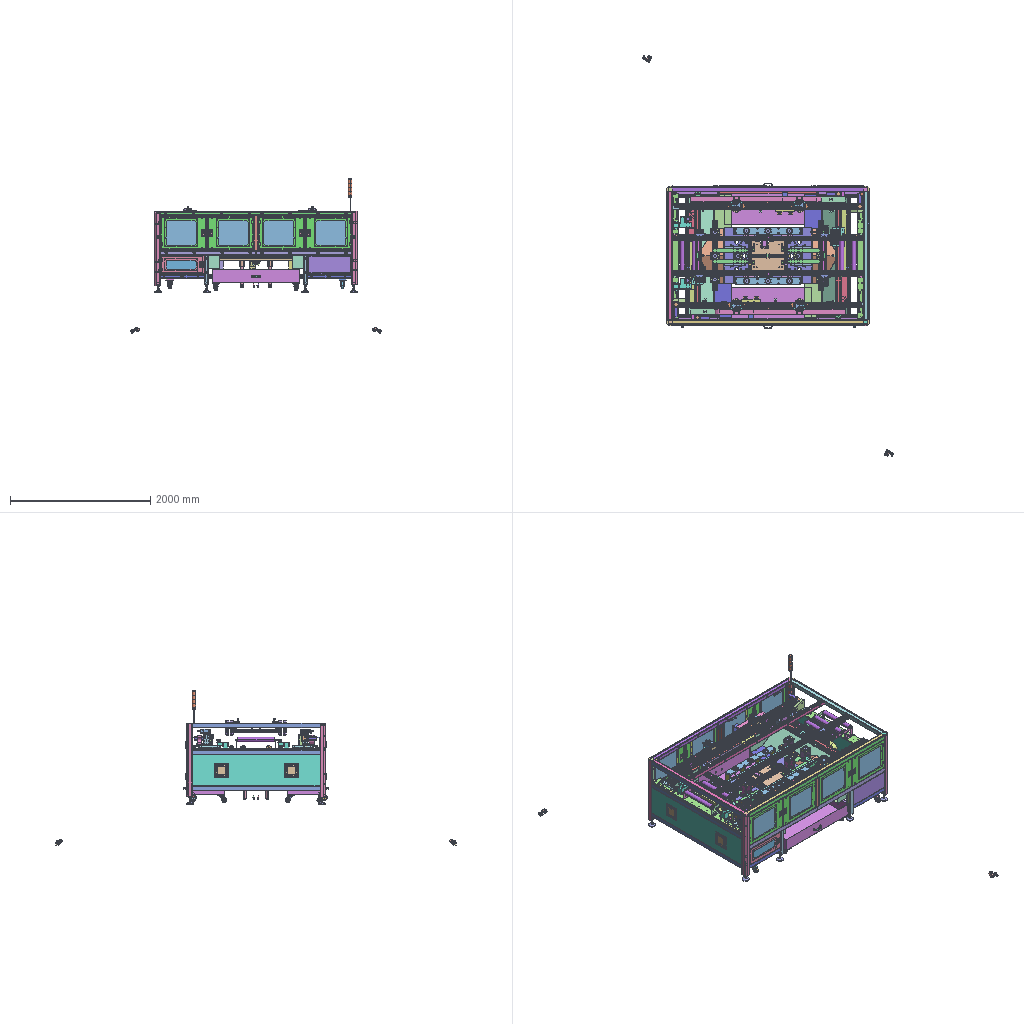Assembly | SolidWorks | 246 different items | 1119 placed | box 3582 x 5733 x 2213 mm
Parts list (item | name | quantity | parent item | size | volume | features):
1 | (subassembly) | x12 | in 4, 42 | 30 x 63 x 50 mm | 11600 mm3 | -
2 | (subassembly) | x4 | in 42 | 650 x 120 x 55.5 mm | 1855069 mm3 | features CompositeCurve 2
3 | (subassembly) | x1 | - | - | 84353797 mm3 | -
4 | (subassembly) | x2 | in 3 | - | 30075054 mm3 | features ReferencePattern 10, LocalLPattern 3, MirrorCompFeat 1
5 | (subassembly) | x2 | in 4 | 249.5 x 142 x 2600 mm | 14332524 mm3 | -
6 | (subassembly) | x2 | in 4 | 270 x 295.093 x 105 mm | 1190493 mm3 | features ReferencePattern 4, MirrorCompFeat 2
7 | (subassembly) | x4 | in 4 | 139.525 x 248.451 x 255.389 mm | 1113097 mm3 | -
8 | (subassembly) | x2 | in 3 | 1950 x 150 x 55.5 mm | 5101027 mm3 | features ReferencePattern 5, LocalLPattern 2, MirrorCompFeat 1
9 | (subassembly) | x2 | in 3 | 410 x 159.5 x 631 mm | 6148104 mm3 | features ReferencePattern 8, LocalLPattern 1, MirrorCompFeat 1
10 | (subassembly) | x2 | in 3 | 182.598 x 320 x 130 mm | 852374 mm3 | features CompositeCurve 6
11 | (subassembly) | x1 | - | - | 89338303 mm3 | features CompositeCurve 5, ReferencePattern 4, LocalLPattern 1
12 | (subassembly) | x1 | - | - | 55171435 mm3 | features ReferencePattern 18, MirrorCompFeat 9
13 | (subassembly) | x2 | in 12 | 953 x 227 x 231.5 mm | 4552776 mm3 | features ReferencePattern 11, MirrorCompFeat 2, CompositeCurve 1, LocalLPattern 1
14 | (subassembly) | x2 | in 12 | 100 x 125 x 230.841 mm | 827561 mm3 | -
15 | (subassembly) | x1 | in 12 | - | 34812843 mm3 | -
16 | (subassembly) | x1 | in 15 | - | 11539429 mm3 | features ReferencePattern 4, MirrorCompFeat 3, CompositeCurve 1, LocalLPattern 1
17 | (subassembly) | x4 | in 16 | 190 x 97 x 61 mm | 476303 mm3 | features CompositeCurve 1
18 | (subassembly) | x1 | in 15 | 1250 x 536.5 x 800 mm | 23012589 mm3 | features ReferencePattern 6, MirrorCompFeat 2, LocalLPattern 1
19 | (subassembly) | x2 | in 12 | 542.5 x 231.5 x 1000 mm | 4307591 mm3 | features ReferencePattern 11, LocalLPattern 2, MirrorCompFeat 2
20 | (subassembly) | x6 | in 19 | 125 x 100 x 191.5 mm | 742164 mm3 | -
21 | (subassembly) | x1 | - | - | 11952575 mm3 | features ReferencePattern 36, MirrorCompFeat 3, CompositeCurve 2, LocalLPattern 2
22 | (subassembly) | x2 | in 11 | 496 x 60 x 123 mm | 328404 mm3 | features MirrorCompFeat 3, ReferencePattern 3
23 | (subassembly) | x4 | in 21 | 110 x 69 x 42 mm | 113289 mm3 | -
24 | (subassembly) | x20 | in 33, 39 | 20.733 x 18.957 x 75.5 mm | 4578 mm3 | -
25 | (subassembly) | x8 | in 11 | 100 x 168 x 100 mm | 182730 mm3 | -
26 | (subassembly) | x8 | in 40 | 100 x 118 x 127 mm | 289275 mm3 | -
27 | (subassembly) | x2 | in 42 | 249.5 x 90 x 1730 mm | 9701440 mm3 | -
28 | (subassembly) | x8 | in 6, 43 | 118 x 54.3 x 21.2 mm | 85401 mm3 | -
29 | (subassembly) | x4 | in 7 | 177 x 112 x 48 mm | 579896 mm3 | features CompositeCurve 1
30 | (subassembly) | x2 | in 10 | 42 x 93.165 x 114.867 mm | 308752 mm3 | -
31 | (subassembly) | x12 | in 13, 19 | 51.5 x 67 x 13 mm | 7718 mm3 | -
32 | (subassembly) | x1 | in 18 | 421 x 93 x 190.924 mm | 447308 mm3 | -
33 | (subassembly) | x8 | in 11 | 670.712 x 493 x 25 mm | 1584341 mm3 | features MirrorCompFeat 1, ReferencePattern 1
34 | (subassembly) | x1 | in 16 | 137.5 x 90 x 275 mm | 2048513 mm3 | -
35 | (subassembly) | x4 | in 21 | 21 x 58.38 x 21 mm | 7646 mm3 | -
36 | (subassembly) | x6 | in 21 | 134.5 x 110 x 44 mm | 443545 mm3 | -
37 | (subassembly) | x4 | in 27, 38 | 60 x 60 x 244.5 mm | 699844 mm3 | -
38 | (subassembly) | x2 | in 5 | 180 x 130 x 249.5 mm | 881824 mm3 | -
39 | (subassembly) | x2 | in 11 | 632.212 x 271 x 25 mm | 870421 mm3 | features MirrorCompFeat 1, ReferencePattern 1
40 | (subassembly) | x2 | in 11 | 1330 x 308 x 617 mm | 5317386 mm3 | features ReferencePattern 3, LocalLPattern 1
41 | (subassembly) | x2 | in 11 | 186.8 x 59 x 30 mm | 74237 mm3 | -
42 | (subassembly) | x2 | - | 3126 x 3821 x 1424 mm | 19246728 mm3 | features ReferencePattern 9, LocalLPattern 2, MirrorCompFeat 1
43 | (subassembly) | x2 | in 42 | 270 x 229 x 105 mm | 1017603 mm3 | features ReferencePattern 4, MirrorCompFeat 2
44 | - | x1 | in 11 | 2850 x 360 x 1986 mm | 11675407 mm3 | features BaseBody 47
45 | - | x2 | in 21 | 80 x 40 x 622 mm | 667832 mm3 | features Fillet 2, Extrusion 1, ICE 1
46 | - | x8 | in 21 | 20 x 22 x 23 mm | 8411 mm3 | features Chamfer 1, Extrusion 1, HoleWzd 1
47 | - | x1 | in 21 | 140 x 163 x 12 mm | 222446 mm3 | features HoleWzd 5, Chamfer 3, Fillet 2, ICE 2, Extrusion 1, LPattern 1, MirrorPattern 1
48 | - | x4 | in 21 | 75 x 32 x 16 mm | 23656 mm3 | features Chamfer 2, HoleWzd 2, Extrusion 1, ICE 1
49 | - | x8 | in 21 | 20 x 10 x 9.5 mm | 1299 mm3 | features ICE 2, Extrusion 1, MirrorPattern 1
50 | - | x1 | in 21 | 130 x 12 x 75 mm | 110369 mm3 | features BaseBody 1
51 | - | x9 | in 21 | 40 x 25 x 18 mm | 14348 mm3 | features Chamfer 2, ICE 2, Extrusion 1, HoleWzd 1
52 | - | x4 | in 21 | 112 x 68 x 12 mm | 60173 mm3 | features HoleWzd 3, Chamfer 1, Cut 1, Extrusion 1, Fillet 1, MirrorPattern 1
53 | - | x1 | in 21 | 140 x 163 x 12 mm | 222446 mm3 | features HoleWzd 5, ICE 4, Chamfer 1, Extrusion 1, Fillet 1
54 | - | x1 | in 21 | 110 x 60 x 137 mm | 135582 mm3 | features HoleWzd 2, EdgeFlange 1, Fillet 1, FlatPattern 1, ICE 1, SMBaseFlange 1, SheetMetal 1
55 | - | x2 | in 11 | 628 x 20 x 273 mm | 459203 mm3 | features ICE 3, MirrorPattern 2, FlatPattern 1, SMBaseFlange 1, SMMiteredFlange 1, SheetMetal 1
56 | - | x4 | in 21 | 25 x 27.5 x 1.5 mm | 706.258 mm3 | features Extrusion 1, Fillet 1, HoleWzd 1
57 | - | x2 | in 21 | 60 x 30 x 2720 mm | 2264041 mm3 | features Cut 2, Extrusion 1
58 | - | x4 | in 23 | 110 x 8 x 42 mm | 33353 mm3 | features HoleWzd 2, MirrorPattern 2, Chamfer 1, Extrusion 1
59 | - | x10 | in 33, 39 | 60 x 94 x 17 mm | 35696 mm3 | features BaseBody 1
60 | - | x1 | in 11 | 52 x 469 x 52 mm | 591292 mm3 | features ICE 1, RefAxis 1, RevCut 1, Revolution 1
61 | - | x3 | in 11 | 204 x 204 x 20 mm | 703498 mm3 | features ICE 2, SweepCut 2, Extrusion 1
62 | - | x6 | in 40 | 140 x 40 x 26 mm | 36488 mm3 | features ICE 3, Fillet 2, Extrusion 1, HoleWzd 1, MirrorPattern 1
63 | - | x8 | in 4, 42 | 48 x 30.5 x 84 mm | 91116 mm3 | features BaseBody 1
64 | - | x2 | in 42 | 617.546 x 830.514 x 284.328 mm | 3734019 mm3 | features ExtruThin 1
65 | - | x12 | in 1 | 12 x 12 x 48 mm | 3806 mm3 | features ICE 2
66 | - | x2 | in 22 | 496 x 60 x 60 mm | 303095 mm3 | features EdgeFlange 2, ICE 2, SMBaseFlange 2, FlatPattern 1, HoleWzd 1, LPattern 1, MirrorSolid 1, SheetMetal 1
67 | - | x4 | in 2 | 23 x 22 x 590 mm | 242690 mm3 | features ICE 2, BaseBody 1, LPattern 1
68 | - | x2 | in 4 | 68 x 132.441 x 1862 mm | 5807055 mm3 | features ExtruThin 1
69 | - | x4 | in 8 | 23 x 22 x 260 mm | 107500 mm3 | features ICE 2, BaseBody 1, HoleWzd 1, LPattern 1
70 | - | x14 | in 13, 14, 20 | 83 x 20.5 x 83 mm | 40041 mm3 | features Revolution 1
71 | - | x4 | in 13 | 23 x 22 x 180 mm | 87654 mm3 | features Extrusion 1, HoleWzd 1, LPattern 1
72 | - | x6 | in 13, 19 | 48 x 34.5 x 84 mm | 100839 mm3 | features BaseBody 1
73 | - | x4 | in 18 | 96 x 96 x 151 mm | 288115 mm3 | features ICE 2, 3DProfileFeature 1, Extrusion 1, HoleWzd 1
74 | - | x1 | in 18 | 53 x 53 x 102 mm | 127493 mm3 | features BaseBody 1
75 | - | x4 | in 18 | 102 x 40 x 56 mm | 73509 mm3 | features ICE 3, Extrusion 1, MirrorPattern 1
76 | - | x2 | in 16 | 95 x 60 x 24.5 mm | 44207 mm3 | features ICE 7, Fillet 3, MirrorPattern 2, Extrusion 1, HoleWzd 1, RefAxis 1
77 | - | x8 | in 22 | 34.18 x 31.5 x 36 mm | 6327 mm3 | features EdgeFlange 2, FlatPattern 1, HoleWzd 1, SMBaseFlange 1, SheetMetal 1
78 | - | x1 | in 16 | 71 x 45 x 19.5 mm | 23170 mm3 | features ICE 7, Fillet 2, MirrorPattern 2, Extrusion 1, HoleWzd 1, RefAxis 1
79 | - | x2 | in 16 | 198.54 x 30 x 1498 mm | 429965 mm3 | features ExtruThin 1
80 | - | x4 | in 12 | 23 x 22 x 445 mm | 217006 mm3 | features Extrusion 1, HoleWzd 1, LPattern 1
81 | - | x2 | in 41 | 165 x 44 x 29 mm | 60919 mm3 | features ICE 15, Extrusion 1, Fillet 1, MirrorPattern 1
82 | - | x4 | in 21 | 70 x 30.5 x 84 mm | 110295 mm3 | features BaseBody 1
83 | - | x4 | in 21 | 23 x 22 x 610 mm | 256299 mm3 | features ICE 3, BaseBody 1, HoleWzd 1, LPattern 1
84 | - | x2 | in 21 | 141 x 60 x 32 mm | 81760 mm3 | features BaseBody 1
85 | - | x40 | in 7, 16, 17, 23 | 9 x 32 x 32 mm | 4178 mm3 | features Revolution 3, CirPattern 1, Fillet 1
86 | - | x8 | in 28 | 110.5 x 54.3 x 21.2 mm | 77984 mm3 | features BaseBody 1
87 | - | x1 | in 32 | 53 x 15.5 x 15.5 mm | 5397 mm3 | features BaseBody 1
88 | - | x8 | in 33 | 664.5 x 493 x 20 mm | 495886 mm3 | features Cut 3, ICE 2, Fillet 1, FlatPattern 1, MirrorPattern 1, SMBaseFlange 1, SMMiteredFlange 1, SheetMetal 1
89 | - | x1 | in 32 | 53 x 15.5 x 15.5 mm | 5397 mm3 | features BaseBody 1
90 | - | x1 | in 32 | 10 x 10 x 24.2 mm | 1321 mm3 | features BaseBody 1
91 | - | x1 | in 32 | 10 x 10 x 24.2 mm | 1321 mm3 | features BaseBody 1
92 | - | x1 | in 32 | 10 x 9.485 x 1.224 mm | 14.034 mm3 | features BaseBody 1
93 | - | x1 | in 32 | 10 x 9.485 x 1.224 mm | 14.034 mm3 | features BaseBody 1
94 | - | x4 | in 35 | 16.166 x 26 x 14 mm | 2413 mm3 | features BaseBody 1
95 | - | x2 | in 30 | 42 x 93 x 87.5 mm | 227496 mm3 | features BaseBody 1
96 | - | x1 | in 32 | 42 x 93 x 112.5 mm | 290888 mm3 | features BaseBody 1
97 | - | x6 | in 36 | 112.5 x 93 x 42 mm | 290420 mm3 | features BaseBody 1
98 | - | x8 | in 28 | 8 x 53 x 20 mm | 7417 mm3 | features BaseBody 1
99 | - | x8 | in 33 | 5 x 400 x 480 mm | 959327 mm3 | features Extrusion 1, Fillet 1, ICE 1
100 | - | x4 | in 35 | 21 x 58.38 x 21 mm | 5233 mm3 | features BaseBody 1
101 | - | x2 | in 30 | 38 x 91 x 102 mm | 81256 mm3 | features BaseBody 1
102 | - | x1 | in 32 | 38 x 91 x 160 mm | 107406 mm3 | features BaseBody 1
103 | - | x6 | in 36 | 115 x 110 x 44 mm | 118873 mm3 | features BaseBody 1
104 | - | x1 | in 32 | 10 x 30.022 x 26 mm | 3164 mm3 | features BaseBody 1
105 | - | x6 | in 36 | 92.5 x 32 x 32 mm | 32646 mm3 | features BaseBody 1
106 | - | x1 | in 32 | 53 x 15.5 x 15.5 mm | 5397 mm3 | features BaseBody 1
107 | - | x6 | in 36 | 25 x 13 x 13 mm | 1601 mm3 | features BaseBody 1
108 | - | x1 | in 32 | 53 x 15.5 x 15.5 mm | 5397 mm3 | features BaseBody 1
109 | - | x1 | in 32 | 53 x 15.5 x 15.5 mm | 5397 mm3 | features BaseBody 1
110 | - | x8 | in 33 | 2 x 400 x 480 mm | 84276 mm3 | features Fillet 2, ICE 2, Extrusion 1
111 | - | x1 | in 32 | 53 x 15.5 x 15.5 mm | 5397 mm3 | features BaseBody 1
112 | - | x4 | in 29 | 112.5 x 112 x 48 mm | 379954 mm3 | features BaseBody 1
113 | - | x4 | in 29 | 177 x 110 x 44 mm | 157829 mm3 | features BaseBody 1
114 | - | x4 | in 29 | 117.5 x 32 x 32 mm | 40502 mm3 | features BaseBody 1
115 | - | x4 | in 29 | 25 x 13 x 13 mm | 1601 mm3 | features BaseBody 1
116 | - | x1 | in 32 | 53 x 15.5 x 15.5 mm | 5397 mm3 | features BaseBody 1
117 | - | x1 | in 32 | 53 x 15.5 x 15.5 mm | 5397 mm3 | features BaseBody 1
118 | - | x12 | in 31 | 10 x 57.8 x 10 mm | 2436 mm3 | features RefAxis 3, 3DProfileFeature 1, ICE 1, Revolution 1
119 | - | x12 | in 31 | 51.5 x 31 x 13 mm | 5282 mm3 | features RefAxis 3, ICE 2, 3DProfileFeature 1, RevCut 1, Revolution 1
120 | - | x4 | in 27, 38 | 44 x 44 x 27 mm | 22442 mm3 | features ICE 4, CirPattern 2, Fillet 2, MirrorPattern 2, Extrusion 1, HoleWzd 1
121 | - | x2 | in 39 | 626 x 271 x 20 mm | 336967 mm3 | features Cut 3, ICE 2, Fillet 1, FlatPattern 1, MirrorPattern 1, SMBaseFlange 1, SMMiteredFlange 1, SheetMetal 1
122 | - | x8 | in 25 | 100 x 168 x 100 mm | 180042 mm3 | features ICE 3, Revolution 1
123 | - | x8 | in 25 | 21 x 10 x 24.249 mm | 2688 mm3 | features Extrusion 1, HoleWzd 1
124 | - | x4 | in 27, 38 | 44 x 44 x 27 mm | 23897 mm3 | features ICE 4, CirPattern 2, Fillet 2, MirrorPattern 2, Extrusion 1, HoleWzd 1
125 | - | x4 | in 37 | 60 x 60 x 155 mm | 420102 mm3 | features ICE 4, HoleWzd 2, MirrorPattern 2, Extrusion 1, Fillet 1
126 | - | x4 | in 37 | 60 x 60 x 119.5 mm | 279742 mm3 | features ICE 11, CirPattern 3, HoleWzd 2, Extrusion 1, Fillet 1
127 | - | x20 | in 24 | 16 x 12 x 60 mm | 2875 mm3 | features Cut 1, FlatPattern 1, Hem 1, SMBaseFlange 1, SheetMetal 1
128 | - | x20 | in 24 | 17.5 x 75.5 x 5 mm | 1703 mm3 | features Sweep 1
129 | - | x8 | in 26 | 94 x 12.5 x 67 mm | 35505 mm3 | features Cut 2, Extrusion 1, Fillet 1, Revolution 1
130 | - | x1 | in 34 | 138 x 102.5 x 90 mm | 973756 mm3 | features ICE 10, Fillet 6, CirPattern 3, HoleWzd 2, Chamfer 1, Extrusion 1
131 | - | x1 | in 34 | 125 x 90 x 174 mm | 1074757 mm3 | features ICE 6, Fillet 2, CirPattern 1, Extrusion 1
132 | - | x2 | in 39 | 5 x 178 x 480 mm | 426527 mm3 | features Extrusion 1, Fillet 1, ICE 1
133 | - | x4 | in 5, 27 | 75 x 16 x 210 mm | 219565 mm3 | features HoleWzd 2, Extrusion 1, LPattern 1, MirrorPattern 1
134 | - | x2 | in 5 | 75 x 75 x 2340 mm | 12326933 mm3 | features ICE 3, Extrusion 1, MirrorPattern 1
135 | - | x2 | in 27 | 75 x 75 x 1465 mm | 7717503 mm3 | features ICE 3, Extrusion 1, MirrorPattern 1
136 | - | x2 | in 5 | 110 x 75 x 80 mm | 456028 mm3 | features HoleWzd 3, ICE 3, Extrusion 1
137 | - | x2 | in 27 | 110 x 75 x 80 mm | 448429 mm3 | features HoleWzd 3, ICE 3, Extrusion 1
138 | - | x4 | in 5, 27 | 75 x 75 x 80 mm | 448174 mm3 | features Extrusion 1, HoleWzd 1
139 | - | x2 | in 27 | 185 x 8 x 90 mm | 84254 mm3 | features ICE 5, HoleWzd 3, Chamfer 2, Extrusion 1, Fillet 1
140 | - | x2 | in 38 | 180 x 130 x 8 mm | 96811 mm3 | features HoleWzd 7, ICE 7, Chamfer 2, Extrusion 1, Fillet 1, LPattern 1
141 | - | x4 | in 27, 38 | 20 x 20 x 1.5 mm | 169.646 mm3 | features Extrusion 1
142 | - | x4 | in 27, 38 | 22 x 22 x 5 mm | 617.009 mm3 | features Chamfer 1, Extrusion 1, ICE 1
143 | - | x2 | in 39 | 2 x 178 x 480 mm | 62076 mm3 | features Fillet 2, ICE 2, Extrusion 1
144 | - | x8 | in 26 | 100 x 10 x 100 mm | 98547 mm3 | features 3DProfileFeature 1, Extrusion 1, HoleWzd 1
145 | - | x8 | in 26 | 74 x 74 x 32 mm | 122167 mm3 | features Fillet 1, Revolution 1
146 | - | x8 | in 26 | 58 x 81 x 70.5 mm | 30390 mm3 | features Cut 4, Fillet 3, Boss 1, Revolution 1
147 | - | x8 | in 26 | 8 x 53 x 8 mm | 2664 mm3 | features Extrusion 1
148 | - | x8 | in 27, 38 | 25 x 25 x 5 mm | 2269 mm3 | features Chamfer 1, Extrusion 1
149 | - | x2 | in 9 | 400 x 136 x 40 mm | 236544 mm3 | features MirrorStock 1
150 | - | x2 | in 9 | 40 x 20 x 4 mm | 2083 mm3 | features MirrorStock 1
151 | - | x2 | in 11 | 1770 x 649.052 x 254.655 mm | 3040079 mm3 | features BaseBody 4
152 | - | x2 | in 40 | 1250 x 190 x 550 mm | 4050815 mm3 | features HoleWzd 3, MirrorPattern 2, EdgeFlange 1, FlatPattern 1, LPattern 1, SMBaseFlange 1, SheetMetal 1, WeldmentFeature 1
153 | - | x2 | in 41 | 139 x 15 x 30 mm | 13318 mm3 | features EdgeFlange 2, Fillet 1, FlatPattern 1, HoleWzd 1, ICE 1, MirrorPattern 1, SMBaseFlange 1, SheetMetal 1
154 | - | x2 | in 42 | 150 x 75 x 92 mm | 232995 mm3 | features HoleWzd 4, ICE 4, Chamfer 1, Extrusion 1
155 | - | x2 | in 42 | 84 x 1425 x 22 mm | 348918 mm3 | features EdgeFlange 1, Fillet 1, FlatPattern 1, HoleWzd 1, SMBaseFlange 1, SheetMetal 1
156 | - | x8 | in 42 | 45 x 65 x 90 mm | 23018 mm3 | features HoleWzd 2, EdgeFlange 1, Fillet 1, FlatPattern 1, ICE 1, MirrorPattern 1, SMBaseFlange 1, SheetMetal 1
157 | - | x2 | in 42 | 193 x 98 x 52 mm | 135822 mm3 | features EdgeFlange 1, FlatPattern 1, ICE 1, SMBaseFlange 1, SheetMetal 1
158 | - | x6 | in 4, 42 | 80 x 29 x 7 mm | 7737 mm3 | features ICE 4, Extrusion 1, MirrorPattern 1
159 | - | x6 | in 4, 42 | 80 x 21 x 12 mm | 13492 mm3 | features ICE 2, Extrusion 1, MirrorPattern 1
160 | - | x6 | in 4, 42 | 42 x 41 x 15 mm | 15925 mm3 | features HoleWzd 3, Chamfer 2, ICE 2, Extrusion 1
161 | - | x6 | in 4, 42 | 40 x 20 x 15 mm | 1805 mm3 | features EdgeFlange 1, Fillet 1, FlatPattern 1, HoleWzd 1, ICE 1, SMBaseFlange 1, SheetMetal 1
162 | - | x4 | in 11 | 80 x 1039 x 80 mm | 334294 mm3 | features FlatPattern 4, EdgeFlange 2, HoleWzd 2, LPattern 2, SMBaseFlange 2, SheetMetal 2, Fillet 1, ICE 1, MirrorSolid 1
163 | - | x6 | in 6, 43 | 110 x 8 x 165 mm | 104521 mm3 | features ICE 3, Chamfer 2, HoleWzd 2, Extrusion 1, Fillet 1
164 | - | x8 | in 6, 43 | 30 x 75 x 6.5 mm | 13862 mm3 | features Chamfer 1, Extrusion 1, HoleWzd 1
165 | - | x8 | in 6, 43 | 105 x 30 x 2 mm | 4885 mm3 | features Chamfer 2, ICE 2, Extrusion 1
166 | - | x2 | in 43 | 270 x 192 x 12 mm | 526570 mm3 | features HoleWzd 8, Chamfer 1, Extrusion 1, Fillet 1, ICE 1, MirrorPattern 1
167 | - | x8 | in 6, 43 | 62 x 75 x 25 mm | 89108 mm3 | features HoleWzd 3, Chamfer 1, Extrusion 1, ICE 1
168 | - | x12 | in 1 | 30 x 48 x 50 mm | 7794 mm3 | features HoleWzd 2, Chamfer 1, EdgeFlange 1, Fillet 1, FlatPattern 1, ICE 1, SMBaseFlange 1, SheetMetal 1
169 | - | x4 | in 2 | 650 x 120 x 16 mm | 1230763 mm3 | features HoleWzd 5, Chamfer 1, Cut 1, Extrusion 1, ICE 1, MirrorPattern 1
170 | - | x16 | in 2, 8 | 50 x 35 x 20 mm | 27074 mm3 | features Chamfer 1, Extrusion 1, HoleWzd 1
171 | - | x16 | in 2, 8 | 40 x 39.5 x 21 mm | 10051 mm3 | features ICE 2, EdgeFlange 1, Fillet 1, FlatPattern 1, SMBaseFlange 1, SheetMetal 1
172 | - | x4 | in 2 | 25 x 25 x 590 mm | 288109 mm3 | features HoleWzd 2, Chamfer 1, Extrusion 1
173 | - | x6 | in 11 | 1828 x 20 x 60 mm | 338800 mm3 | features FlatPattern 6, SMBaseFlange 3, SheetMetal 3, EdgeFlange 2, HoleWzd 2, MirrorSolid 2, ICE 1, LPattern 1
174 | - | x8 | in 2, 21 | 585 x 27.5 x 1.2 mm | 19258 mm3 | features Extrusion 1, HoleWzd 1
175 | - | x2 | in 4 | 80 x 80 x 2500 mm | 4298649 mm3 | features HoleWzd 3, ICE 3, MirrorPattern 3, Fillet 2, Extrusion 1
176 | - | x4 | in 4 | 160 x 172 x 80 mm | 351912 mm3 | features HoleWzd 7, ICE 4, Chamfer 3, Extrusion 1, Fillet 1
177 | - | x2 | in 6 | 270 x 255 x 12 mm | 594940 mm3 | features HoleWzd 7, Chamfer 2, Extrusion 1, Fillet 1, ICE 1, MirrorPattern 1
178 | - | x8 | in 4 | 105 x 80 x 10 mm | 64132 mm3 | features HoleWzd 2, ICE 2, Chamfer 1, Extrusion 1, LPattern 1
179 | - | x2 | in 4 | 2200 x 22 x 84 mm | 538758 mm3 | features EdgeFlange 1, FlatPattern 1, HoleWzd 1, SMBaseFlange 1, SheetMetal 1
180 | - | x10 | in 4 | 45 x 75 x 50 mm | 18329 mm3 | features HoleWzd 2, EdgeFlange 1, Fillet 1, FlatPattern 1, ICE 1, MirrorPattern 1, SMBaseFlange 1, SheetMetal 1
181 | - | x2 | in 4 | 140 x 80 x 145 mm | 202654 mm3 | features EdgeFlange 2, HoleWzd 2, Chamfer 1, FlatPattern 1, SMBaseFlange 1, SheetMetal 1
182 | - | x2 | in 4 | 188 x 138 x 52 mm | 149512 mm3 | features ICE 3, EdgeFlange 2, FlatPattern 1, SMBaseFlange 1, SheetMetal 1
183 | - | x4 | in 7 | 165 x 10 x 130 mm | 178230 mm3 | features Chamfer 3, ICE 2, Extrusion 1, HoleWzd 1, MirrorPattern 1
184 | - | x4 | in 11 | 415 x 20 x 60 mm | 80765 mm3 | features FlatPattern 3, EdgeFlange 2, SMBaseFlange 2, SheetMetal 2, HoleWzd 1, ICE 1, LPattern 1, MirrorSolid 1
185 | - | x4 | in 7 | 110 x 77 x 43 mm | 86421 mm3 | features HoleWzd 2, ICE 2, Chamfer 1, Extrusion 1
186 | - | x8 | in 7, 23 | 40 x 40 x 41 mm | 32585 mm3 | features Chamfer 1, Extrusion 1, ICE 1, MirrorPattern 1
187 | - | x8 | in 7, 23 | 40 x 61 x 40 mm | 20124 mm3 | features Chamfer 2, ICE 2, Extrusion 1, HoleWzd 1, RevCut 1
188 | - | x4 | in 7 | 250 x 80 x 10 mm | 195481 mm3 | features HoleWzd 3, MirrorPattern 3, Chamfer 1, Extrusion 1
189 | - | x4 | in 7 | 80 x 19 x 1 mm | 1481 mm3 | features Extrusion 1, HoleWzd 1
190 | - | x4 | in 8 | 1950 x 150 x 16 mm | 4450489 mm3 | features HoleWzd 12, MirrorPattern 7, LPattern 5, Fillet 3, Cut 1, Extrusion 1
191 | - | x4 | in 8 | 25 x 25 x 280 mm | 135760 mm3 | features HoleWzd 2, Chamfer 1, Extrusion 1
192 | - | x4 | in 8 | 300 x 26 x 1 mm | 7761 mm3 | features Extrusion 1, HoleWzd 1
193 | - | x6 | in 9 | 65 x 65 x 575 mm | 1777108 mm3 | features ICE 2, Extrusion 1, Fillet 1, MirrorPattern 1
194 | - | x2 | in 9 | 400 x 136 x 40 mm | 236544 mm3 | features Fillet 5, HoleWzd 3, LPattern 3, ICE 2, Chamfer 1, EdgeFlange 1, FlatPattern 1, SMBaseFlange 1, SheetMetal 1
195 | - | x4 | in 11 | 628 x 20 x 60 mm | 120616 mm3 | features FlatPattern 4, EdgeFlange 2, SMBaseFlange 2, SheetMetal 2, HoleWzd 1, ICE 1, LPattern 1, MirrorSolid 1
196 | - | x10 | in 9 | 40 x 20 x 4 mm | 2083 mm3 | features ICE 3, Chamfer 1, Extrusion 1, Fillet 1, LPattern 1
197 | - | x2 | in 9 | 40 x 40 x 551 mm | 331194 mm3 | features HoleWzd 3, Fillet 2, ICE 2, CirPattern 1, Extrusion 1, LPattern 1
198 | - | x2 | in 10 | 176 x 260 x 130 mm | 504941 mm3 | features ICE 9, HoleWzd 4, Fillet 3, Extrusion 1, MirrorPattern 1
199 | - | x4 | in 10 | 140.785 x 42 x 17.598 mm | 17021 mm3 | features EdgeFlange 1, Fillet 1, FlatPattern 1, HoleWzd 1, SMBaseFlange 1, SheetMetal 1
200 | - | x2 | in 10 | 80 x 30 x 2 mm | 4639 mm3 | features HoleWzd 2, Fillet 1, FlatPattern 1, SMBaseFlange 1, SheetMetal 1
201 | - | x5 | in 12 | 300 x 26 x 1 mm | 7761 mm3 | features Extrusion 1, HoleWzd 1
202 | - | x4 | in 12 | 100 x 19 x 1 mm | 1861 mm3 | features Extrusion 1, HoleWzd 1
203 | - | x2 | in 13 | 100 x 925 x 20 mm | 1485141 mm3 | features HoleWzd 3, ICE 2, Extrusion 1, Fillet 1, MirrorPattern 1
204 | - | x8 | in 13 | 153.5 x 80 x 15 mm | 173749 mm3 | features HoleWzd 2, Chamfer 1, Extrusion 1, MirrorPattern 1
205 | - | x2 | in 13 | 950 x 185 x 15 mm | 1463196 mm3 | features HoleWzd 5, MirrorPattern 3, Chamfer 2, Fillet 2, ICE 2, Extrusion 1
206 | - | x4 | in 11 | 1364 x 20 x 60 mm | 253951 mm3 | features FlatPattern 5, EdgeFlange 2, SMBaseFlange 2, SheetMetal 2, HoleWzd 1, ICE 1, LPattern 1, MirrorSolid 1
207 | - | x14 | in 13, 14, 20 | 112 x 35 x 80 mm | 84771 mm3 | features ICE 3, HoleWzd 2, Chamfer 1, Extrusion 1, RevCut 1
208 | - | x14 | in 13, 14, 20 | 20 x 20 x 80.5 mm | 19122 mm3 | features ICE 3, HoleWzd 2, Chamfer 1, Extrusion 1, MirrorPattern 1, RevCut 1
209 | - | x16 | in 12, 13 | 23 x 22 x 20 mm | 8558 mm3 | features Chamfer 1, Extrusion 1, HoleWzd 1
210 | - | x12 | in 13, 19 | 65 x 37 x 16 mm | 21186 mm3 | features HoleWzd 3, Chamfer 1, Extrusion 1, ICE 1
211 | - | x16 | in 13, 19 | 20 x 11 x 9.5 mm | 1453 mm3 | features ICE 2, Extrusion 1, MirrorPattern 1
212 | - | x8 | in 13, 19 | 25 x 50.651 x 1.5 mm | 1403 mm3 | features Extrusion 1, Fillet 1, HoleWzd 1
213 | - | x8 | in 14, 20 | 100 x 125 x 20 mm | 122158 mm3 | features HoleWzd 2, Extrusion 1, Fillet 1, ICE 1, MirrorPattern 1
214 | - | x4 | in 14 | 193.5 x 80 x 15 mm | 211454 mm3 | features HoleWzd 4, Chamfer 1, Extrusion 1, ICE 1
215 | - | x8 | in 14, 20 | 125 x 80 x 15 mm | 138563 mm3 | features HoleWzd 2, Chamfer 1, Extrusion 1
216 | - | x4 | in 15 | 75 x 45 x 65 mm | 65207 mm3 | features ICE 2, Chamfer 1, Extrusion 1, HoleWzd 1
217 | - | x2 | in 11 | 1828 x 20 x 453 mm | 1833705 mm3 | features ICE 3, MirrorPattern 2, FlatPattern 1, SMBaseFlange 1, SMMiteredFlange 1, SheetMetal 1
218 | - | x1 | in 16 | 80 x 545 x 1250 mm | 4052251 mm3 | features BaseBody 5
219 | - | x2 | in 16 | 250 x 170 x 10 mm | 343286 mm3 | features HoleWzd 3, ICE 2, Extrusion 1, Fillet 1, LPattern 1, MirrorPattern 1
220 | - | x1 | in 16 | 37 x 115 x 115 mm | 322702 mm3 | features ICE 6, Fillet 2, HoleWzd 2, MirrorPattern 2, CirPattern 1, Extrusion 1
221 | - | x4 | in 16 | 60 x 15 x 15 mm | 9274 mm3 | features MirrorPattern 2, Chamfer 1, Extrusion 1, ICE 1, RevCut 1
222 | - | x4 | in 16 | 60 x 60 x 35 mm | 54034 mm3 | features Chamfer 1, Extrusion 1, ICE 1, MirrorPattern 1
223 | - | x1 | in 16 | 250 x 170 x 10 mm | 336944 mm3 | features HoleWzd 3, LPattern 3, ICE 2, Extrusion 1, Fillet 1, MirrorPattern 1
224 | - | x1 | in 16 | 250 x 170 x 10 mm | 346172 mm3 | features HoleWzd 3, ICE 2, Extrusion 1, Fillet 1, LPattern 1, MirrorPattern 1
225 | - | x1 | in 16 | 115 x 115 x 37 mm | 332155 mm3 | features ICE 7, MirrorPattern 4, HoleWzd 2, CirPattern 1, Extrusion 1, RefAxis 1
226 | - | x8 | in 17 | 180 x 76 x 10 mm | 125449 mm3 | features HoleWzd 2, Chamfer 1, Extrusion 1, ICE 1, LPattern 1, MirrorPattern 1
227 | - | x4 | in 17 | 37 x 97 x 97 mm | 204655 mm3 | features ICE 6, MirrorPattern 3, Fillet 2, CirPattern 1, Extrusion 1
228 | - | x4 | in 11 | 1364 x 20 x 68 mm | 272677 mm3 | features FlatPattern 5, EdgeFlange 2, SMBaseFlange 2, SheetMetal 2, HoleWzd 1, ICE 1, LPattern 1, MirrorSolid 1
229 | - | x4 | in 17 | 17 x 17 x 60 mm | 12395 mm3 | features MirrorPattern 2, Chamfer 1, Extrusion 1, HoleWzd 1, ICE 1, RevCut 1
230 | - | x1 | in 16 | 609 x 25 x 25 mm | 250736 mm3 | features ICE 3, Chamfer 2, LPattern 2, RevCut 2, Extrusion 1, Fillet 1
231 | - | x1 | in 18 | 545 x 16 x 465 mm | 3609981 mm3 | features HoleWzd 5, MirrorPattern 5, ICE 4, Chamfer 2, Extrusion 1, Fillet 1
232 | - | x1 | in 18 | 58 x 15 x 90 mm | 71339 mm3 | features HoleWzd 2, Chamfer 1, Extrusion 1
233 | - | x1 | in 18 | 100 x 170 x 61 mm | 189727 mm3 | features Fillet 2, HoleWzd 2, Chamfer 1, Extrusion 1, ICE 1
234 | - | x4 | in 18 | 40 x 40 x 520 mm | 650025 mm3 | features Chamfer 2, HoleWzd 2, Extrusion 1
235 | - | x1 | in 18 | 1250 x 16 x 800 mm | 14520143 mm3 | features MirrorPattern 11, HoleWzd 10, LPattern 5, ICE 4, Chamfer 1, Extrusion 1
236 | - | x2 | in 19 | 80 x 40 x 1000 mm | 1063867 mm3 | features Fillet 2, Extrusion 1
237 | - | x12 | in 20 | 153.5 x 80 x 15 mm | 168755 mm3 | features HoleWzd 2, Chamfer 1, Extrusion 1, ICE 1, MirrorPattern 1
238 | - | x4 | in 19 | 520 x 12 x 65 mm | 396078 mm3 | features HoleWzd 7, Chamfer 1, Extrusion 1, LPattern 1
239 | - | x1 | in 11 | - | 30695338 mm3 | features BaseBody 135
240 | 框架MGPM25-50_0_0_0_ (subassembly) | x1 | - | - | - | -
241 | 框架Mirror气缸FixedPlate 992 | x1 | - | - | - | -
242 | 框架Mirror滑台气缸调节Plate | x1 | - | - | - | -
243 | 框架Mirror短边归正Plate 2334 | x1 | - | - | - | -
244 | 框架Mirror销块1 | x1 | - | - | - | -
245 | 框架Mirror阻挡气缸安装Plate 1 | x1 | - | - | - | -
246 | Mirror短边滑台连接Plate | x1 | - | - | - | -
Mates (type | each side: item.copy, entity, surface, feature), first 324 of 699 lines:
In the top assembly
Coincident | assembly face | assembly face | 14 times
Width | 84.1 face plane 输入1 | 84.1 face plane 输入1 | assembly face | assembly face
Width | 84.2 face plane 输入1 | 84.2 face plane 输入1 | assembly face | assembly face
Coincident | assembly face | 174.1 face plane Boss-Extrude 1
Width | 174.1 face plane Boss-Extrude 1 | 174.1 face plane Boss-Extrude 1 | assembly face | assembly face
Width | 174.2 face plane Boss-Extrude 1 | 174.2 face plane Boss-Extrude 1 | assembly face | assembly face
DistanceDim | assembly face | assembly face | 2 times
Coincident | assembly face | 57.1 face plane Extrude 1 | 2 times
DistanceDim | 57.1 face plane Extrude 1 | assembly face
DistanceDim | 46.1 face plane Boss-Extrude 1 | assembly face
Coincident | assembly face | 57.2 face plane Extrude 1
DistanceDim | 46.2 face plane Boss-Extrude 1 | assembly face
Concentric | assembly face | assembly face | 14 times
Concentric | assembly face | assembly select_type:0 | 4 times
Width | assembly face | assembly face | assembly face | assembly face
Coincident | 239.1 face plane 框架670-5-solid1 | 169.1 face plane Boss-Extrude 1
Concentric | 239.1 face cylinder 框架670-5-solid1 | 169.1 face cylinder M8 六角凹头Screw的柱形沉头Hole 1 | 2 times
Coincident | 239.1 face plane 框架1950-2-solid1 | 190.1 face plane Boss-Extrude 2
Concentric | 239.1 face cylinder 框架1950-2-solid1 | 190.1 face cylinder LPattern 4
Concentric | 239.1 face cylinder 框架1950-2-solid1 | 190.1 face cylinder LPattern 5
In subassembly 42
Coincident | 138.1 face plane Boss-Extrude 1 | 154.1 face plane Boss-Extrude 1 | 2 times
Coincident | 138.1 face plane Boss-Extrude 1 | 154.1 face plane Boss-Extrude 2
Concentric | 138.1 face cylinder M6 Tapped Hole 2 | 154.1 face cylinder Ø7.0 (7) DiameterHole 1
DistanceDim | 155.1 face plane Edge-Flange 1 | 137.1 face plane Boss-Extrude 1
Coincident | 135.1 face plane Boss-Extrude 1 | 156.1 face plane Edge-Flange 1
DistanceDim | 135.1 face plane Boss-Extrude 1 | 156.1 face plane Edge-Flange 1
Coincident | 133.1 face plane Boss-Extrude 1 | 166.1 face plane Boss-Extrude 1
DistanceDim | 166.1 face plane Boss-Extrude 1 | 133.1 face plane Boss-Extrude 1
Coincident | 133.1 plane | 166.1 plane
Coincident | 135.1 face plane Boss-Extrude 1 | 168.1 face plane Base-Flange 1 | 2 times
Width | 158.1 face plane Boss-Extrude 1 | 158.1 face plane Boss-Extrude 1 | 135.1 face plane Boss-Extrude 1 | 135.1 face plane Boss-Extrude 1
Concentric | 154.1 face cylinder M6 六角凹头Screw的柱形沉头Hole 1 | 63.1 face cylinder 输入1 | 2 times
Coincident | 154.1 face plane Cut-Extrude 1 | 63.1 face plane 输入1
Coincident | 154.1 face plane Cut-Extrude 2 | 160.1 face plane Boss-Extrude 1
DistanceDim | 160.1 face plane Boss-Extrude 1 | 154.1 face plane Boss-Extrude 1 | 2 times
Coincident | 154.1 face plane Cut-Extrude 2 | 161.1 face plane Edge-Flange 1
Coincident | 154.1 face plane Boss-Extrude 1 | 161.1 face plane Base-Flange 1
DistanceDim | 154.1 face plane Boss-Extrude 1 | 161.1 face plane Edge-Flange 1
Coincident | 166.1 face plane Boss-Extrude 1 | 158.1 face plane Boss-Extrude 1
Coincident | 166.1 face plane Boss-Extrude 1 | 159.1 face plane Boss-Extrude 1 | 2 times
Concentric | 155.1 face cylinder Ø5.5 (5.5) DiameterHole 1 | 156.1 face cylinder M5 Tapped Hole 1
Coincident | 155.1 face plane Base-Flange 1 | 156.1 face plane Base-Flange 1
Coincident | 158.1 face plane Boss-Extrude 1 | 159.1 face plane Boss-Extrude 1 | 2 times
Coincident | 139.1 face plane Boss-Extrude 1 | 157.1 face plane Edge-Flange 1
Concentric | 139.1 face cylinder M4 Tapped Hole 1 | 157.1 face cylinder Cut-Extrude 1
In subassembly 1
DistanceDim | 168.2 face plane Edge-Flange 1 | 65.1 face plane Boss-Extrude 1
Concentric | 168.2 face cylinder Cut-Extrude 2 | 65.1 face cylinder Boss-Extrude 2
In subassembly 2
Coincident | 169.2 face plane Boss-Extrude 1 | 67.1 face plane 输入1
Concentric | 169.2 face cylinder M6 Tapped Hole 1 | 67.1 face cylinder 输入1 | 2 times
Coincident | 169.2 face plane Boss-Extrude 1 | 170.1 face plane Boss-Extrude 1
Concentric | 169.2 edge | 170.1 face cylinder M8 六角凹头Screw的柱形沉头Hole 1 | 2 times
Coincident | 169.2 face plane Boss-Extrude 1 | 170.2 face plane Boss-Extrude 1
Concentric | 169.2 face cylinder M8 Tapped Hole 1 | 170.2 face cylinder M8 六角凹头Screw的柱形沉头Hole 1 | 2 times
Coincident | 169.2 face plane Boss-Extrude 1 | 171.1 face plane Base-Flange 1
DistanceDim | 171.1 plane | 169.2 face plane Boss-Extrude 1
Width | 171.1 face plane Edge-Flange 1 | 171.2 face plane Edge-Flange 1 | 170.1 face plane Boss-Extrude 1 | 170.2 face plane Boss-Extrude 1
Concentric | 171.1 face cylinder Cut-Extrude 1 | 171.2 face cylinder Cut-Extrude 1
DistanceDim | 171.1 face plane Edge-Flange 1 | 171.2 face plane Edge-Flange 1
Coincident | 171.1 face plane Edge-Flange 1 | 172.1 face plane Boss-Extrude 1
Concentric | 171.1 face cylinder Cut-Extrude 1 | 172.1 face cylinder Boss-Extrude 1
Coincident | 169.2 face plane Boss-Extrude 1 | 174.3 face plane Boss-Extrude 1
Width | 174.3 face plane Boss-Extrude 1 | 174.3 face plane Boss-Extrude 1 | 171.2 face plane Edge-Flange 1 | 171.1 face plane Edge-Flange 1
Coincident | 169.2 face plane Cut-Extrude 1 | 174.3 face plane Boss-Extrude 1
In subassembly 27
Coincident | 135.2 face plane Boss-Extrude 1 | 137.2 face plane Boss-Extrude 1 | 3 times
Coincident | 135.2 face plane Boss-Extrude 1 | 138.2 face plane Boss-Extrude 1 | 3 times
Coincident | 133.2 edge | 135.2 edge
Coincident | 133.2 face plane Boss-Extrude 1 | 135.2 face plane Boss-Extrude 1
Concentric | 139.2 face cylinder Cut-Extrude 8 | 126.1 face cylinder Cut-Extrude 2
Concentric | 139.2 face cylinder M5 Tapped Hole 1 | 126.1 face cylinder Cut-Extrude 6
Concentric | 139.2 face cylinder M5 Tapped Hole 1 | 126.1 face cylinder CirPattern 1
Coincident | 139.2 face plane Boss-Extrude 1 | 126.1 face plane 第二段
Concentric | 139.2 face cylinder Cut-Extrude 9 | 120.1 face cylinder Cut-Extrude 3
Concentric | 139.2 face cylinder Cut-Extrude 9 | 142.1 face cylinder Boss-Extrude 1
Parallel | 139.2 face plane Cut-Extrude 7 | 120.1 plane
Coincident | 141.1 face plane Boss-Extrude 1 | 126.1 face plane Cut-Extrude 2
Concentric | 141.1 face cylinder Boss-Extrude 1 | 126.1 face cylinder Cut-Extrude 2
Coincident | 141.1 face plane Boss-Extrude 1 | 124.1 face plane Cut-Extrude 2
Concentric | 126.1 face cylinder Cut-Extrude 2 | 124.1 face cylinder Cut-Extrude 3
Coincident | 126.1 face plane 第一段 | 148.1 face plane Boss-Extrude 1
Concentric | 126.1 face cylinder M5 Tapped Hole 1 | 148.1 face cylinder Boss-Extrude 1
Coincident | 120.1 face plane Mirror 2 | 142.1 face plane Boss-Extrude 1
Concentric | 120.1 face cylinder Cut-Extrude 3 | 148.2 face cylinder Boss-Extrude 1
Coincident | 120.1 face plane Cut-Extrude 2 | 148.2 face plane Boss-Extrude 1
Coincident | 137.2 face plane Boss-Extrude 1 | 139.2 face plane Boss-Extrude 1
Concentric | 137.2 face cylinder Boss-Extrude 3 | 139.2 face cylinder Cut-Extrude 9
Coincident | 137.2 face plane Boss-Extrude 1 | 139.2 face plane Cut-Extrude 7
In subassembly 37
Concentric | 126.2 face cylinder Cut-Extrude 15 | 125.1 face cylinder Boss-Extrude 3
Concentric | 126.2 face cylinder CirPattern 3 | 125.1 face cylinder Ø4.5 (4.5) DiameterHole 1 | 2 times
Coincident | 126.2 face plane 第三段 | 125.1 face plane Boss-Extrude 1
In subassembly 43
Coincident | 163.1 face plane Boss-Extrude 1 | 166.2 face plane Boss-Extrude 1
Concentric | 163.1 face cone M8 六角凹锥坑Screw的锥形沉头Hole 1 | 166.2 face cylinder M8 Tapped Hole 1
Coincident | 164.1 face plane Boss-Extrude 1 | 165.1 face plane Boss-Extrude 1
Coincident | 165.1 face plane Boss-Extrude 1 | 167.1 face plane Cut-Extrude 1 | 2 times
Concentric | 165.1 face cylinder Cut-Extrude 1 | 167.1 face cylinder M6 Tapped Hole 2
Concentric | 164.1 face cylinder Ø7.0 (7) DiameterHole 1 | 167.1 face cylinder M6 Tapped Hole 2 | 2 times
In subassembly 12
Concentric | 12.1 face | 234.1 face cylinder Boss-Extrude 1
Coincident | 80.1 face plane Boss-Extrude 1 | 209.1 face plane Boss-Extrude 1 | 3 times
Coincident | 80.1 face plane Boss-Extrude 1 | 209.2 face plane Boss-Extrude 1 | 3 times
Coincident | 12.1 face | 80.2 face plane Boss-Extrude 1 | 2 times
DistanceDim | 201.1 face plane Boss-Extrude 1 | 238.1 face plane Boss-Extrude 1
Coincident | 12.1 face | 205.1 face plane Boss-Extrude 1
Coincident | 12.1 face | 215.1 face plane Boss-Extrude 1
Concentric | 12.1 face | 215.1 face cylinder M6 六角凹头Screw的柱形沉头Hole 1 | 2 times
DistanceDim | 12.1 face | 213.1 face plane Boss-Extrude 1
Coincident | 12.1 face | 80.1 face plane Boss-Extrude 1
Width | 238.1 face plane Boss-Extrude 1 | 238.2 face plane Boss-Extrude 1 | 12.1 face | 12.1 face
Coincident | 12.1 face | 201.1 face plane Boss-Extrude 1 | 2 times
Coincident | 12.1 face | 71.1 face plane Boss-Extrude 1
Coincident | 12.1 face | 209.3 face plane Boss-Extrude 1
Width | 205.2 face plane Boss-Extrude 1 | 205.2 face plane Boss-Extrude 1 | 12.1 face | 12.1 face
Coincident | 12.1 face | 202.1 face plane Boss-Extrude 1 | 2 times
DistanceDim | 202.1 face plane Boss-Extrude 1 | 12.1 face
In subassembly 15
Coincident | 231.1 face plane Boss-Extrude 1 | 216.1 face plane Boss-Extrude 1
Slot | 216.1 face plane Cut-Extrude 1 | 231.1 face cylinder Mirror 2 | 2 times
Coincident | 231.1 face plane Boss-Extrude 1 | 216.2 face plane Boss-Extrude 1
Slot | 231.1 face cylinder Mirror 3 | 216.2 face plane Cut-Extrude 1
Slot | 216.2 face plane Cut-Extrude 1 | 231.1 face cylinder Mirror 3
Coincident | 216.1 face plane Boss-Extrude 1 | 216.2 face plane Boss-Extrude 1
Coincident | 231.1 face plane Boss-Extrude 1 | 216.3 face plane Boss-Extrude 1
Slot | 216.3 face plane Cut-Extrude 1 | 231.1 face cylinder M8 Tapped Hole 2 | 2 times
Coincident | 231.1 face plane Boss-Extrude 1 | 216.4 face plane Boss-Extrude 1
Slot | 216.4 face plane Cut-Extrude 1 | 231.1 face cylinder Mirror 3
Slot | 231.1 face cylinder Mirror 3 | 216.4 face plane Cut-Extrude 1
Coincident | 216.3 face plane Boss-Extrude 1 | 216.4 face plane Boss-Extrude 1
DistanceDim | 216.1 face plane Boss-Extrude 1 | 216.3 face plane Boss-Extrude 1
Coincident | 216.1 face plane Boss-Extrude 1 | 15.1 face
DistanceDim | 216.1 face plane Boss-Extrude 1 | 15.1 face
Width | 216.1 face plane Boss-Extrude 1 | 216.2 face plane Boss-Extrude 1 | 15.1 face | 15.1 face
Coincident | 231.1 face plane Boss-Extrude 1 | 15.1 face
In subassembly 18
Concentric | 231.2 face cylinder Ø9.0 (9) DiameterHole 1 | 232.1 face cylinder M8 Tapped Hole 1 | 2 times
Coincident | 231.2 face plane Boss-Extrude 1 | 232.1 face plane Boss-Extrude 1
Coincident | 232.1 face plane Boss-Extrude 1 | 74.1 face plane 输入1
Concentric | 75.1 face cylinder Cut-Extrude 1 | 231.2 face cylinder M10 六角凹头Screw的柱形沉头Hole 1
Coincident | 231.2 face plane Boss-Extrude 1 | 75.1 face plane Boss-Extrude 1
Parallel | 231.2 face plane Boss-Extrude 1 | 75.1 face plane Boss-Extrude 2
Concentric | 234.2 face cylinder Boss-Extrude 1 | 75.1 face cylinder Boss-Extrude 1
Coincident | 231.2 face plane Boss-Extrude 1 | 234.2 face plane Boss-Extrude 1
DistanceDim | 233.1 face plane Boss-Extrude 1 | 231.2 face plane Boss-Extrude 1
Concentric | 233.1 face cylinder Cut-Extrude 1 | 74.1 face cylinder 输入1
Concentric | 231.2 face cylinder Cut-Extrude 10 | 74.1 face cylinder 输入1
Parallel | 231.2 face plane Cut-Extrude 1 | 233.1 face plane Boss-Extrude 1
Concentric | 234.2 face cylinder Boss-Extrude 1 | 73.1 face cylinder Extrude 2
Concentric | 234.3 face cylinder Boss-Extrude 1 | 73.2 face cylinder Extrude 2
Concentric | 234.4 face cylinder Boss-Extrude 1 | 73.3 face cylinder Extrude 2
Concentric | 234.5 face cylinder Boss-Extrude 1 | 73.4 face cylinder Extrude 2
Coincident | 235.1 face plane Boss-Extrude 1 | 233.1 face plane Boss-Extrude 1
Parallel | 234.4 face cylinder Boss-Extrude 1 | 235.1 face cylinder Cut-Extrude 4
Concentric | 235.1 face cylinder Cut-Extrude 4 | 234.4 face cylinder Boss-Extrude 1
Coincident | 235.1 face plane Boss-Extrude 1 | 73.1 face plane Extrude 1
Concentric | 235.1 face cylinder Mirror 6 | 73.1 face cylinder Extrude 1
Concentric | 235.1 face cylinder LPattern 2 | 73.1 face cylinder M8 六角凹头Screw的柱形沉头Hole 1
Concentric | 235.1 face cylinder LPattern 3 | 73.2 face cylinder M8 六角凹头Screw的柱形沉头Hole 1
Coincident | 235.1 face plane Boss-Extrude 1 | 73.2 face plane Extrude 1
Concentric | 235.1 face cylinder M8 Tapped Hole 1 | 73.3 face cylinder M8 六角凹头Screw的柱形沉头Hole 1
Coincident | 235.1 face plane Boss-Extrude 1 | 73.3 face plane Extrude 1
Concentric | 235.1 face cylinder LPattern 3 | 73.4 face cylinder M8 六角凹头Screw的柱形沉头Hole 1
Coincident | 235.1 face plane Boss-Extrude 1 | 73.4 face plane Extrude 1
In subassembly 16
Coincident | 16.1 face | 226.1 face plane Boss-Extrude 1 | 2 times
Coincident | 16.1 face | 226.2 face plane Boss-Extrude 1 | 2 times
Coincident | 16.1 face | 226.3 face plane Boss-Extrude 1
Coincident | 16.1 face | 226.4 face plane Boss-Extrude 1
Coincident | 16.1 face | 226.5 face plane Boss-Extrude 1
Coincident | 16.1 face | 226.6 face plane Boss-Extrude 1
DistanceDim | 16.1 face | 229.1 face plane Mirror 1
DistanceDim | 16.1 face | 229.2 face plane Cut-Extrude 1
DistanceDim | 16.1 face | 229.3 face plane Cut-Extrude 1
DistanceDim | 16.1 face | 229.4 face plane Mirror 1
In subassembly 34
Concentric | 131.1 face cylinder Boss-Extrude 4 | 130.1 face cylinder Cut-Extrude 3
Concentric | 131.1 face cylinder CirPattern 1 | 130.1 face cylinder M6 Tapped Hole 1
Coincident | 131.1 face plane Boss-Extrude 1 | 130.1 face plane Boss-Extrude 1
In subassembly 17
Coincident | 226.7 face plane Boss-Extrude 1 | 226.8 face plane Boss-Extrude 1 | 2 times
DistanceDim | 226.8 face plane Boss-Extrude 1 | 226.7 face plane Boss-Extrude 1
Concentric | 227.1 face cylinder Cut-Extrude 1 | 229.5 face cylinder Boss-Extrude 1
Width | 226.8 face plane Boss-Extrude 1 | 226.7 face plane Boss-Extrude 1 | 227.1 face plane Mirror 2 | 227.1 face plane Boss-Extrude 3
Coincident | 226.8 face plane Cut-Extrude 1 | 229.5 face plane Mirror 1
DistanceDim | 229.5 face plane Mirror 1 | 226.8 face plane Boss-Extrude 1
Parallel | 226.8 face plane Boss-Extrude 1 | 227.1 plane
Concentric | 229.5 face cylinder Boss-Extrude 1 | 85.1 face cylinder Revolve2
Coincident | 227.1 face plane Mirror 3 | 85.1 face plane Revolve3
Concentric | 229.5 face cylinder Boss-Extrude 1 | 85.2 face cylinder Revolve3
Coincident | 227.1 face plane Cut-Extrude 2 | 85.2 face plane Revolve3
Coincident | 229.5 edge | 85.2 face plane Revolve2
In subassembly 14
Coincident | 213.2 face plane Boss-Extrude 1 | 214.1 face plane Boss-Extrude 1
Concentric | 213.2 face cylinder Mirror 2 | 214.1 face cylinder M8 Tapped Hole 2 | 2 times
Coincident | 213.2 face plane Boss-Extrude 1 | 214.2 face plane Boss-Extrude 1
Concentric | 213.2 face cylinder M8 六角凹头Screw的柱形沉头Hole 1 | 214.2 face cylinder M8 Tapped Hole 2 | 2 times
Concentric | 214.1 face cylinder M8 Tapped Hole 1 | 215.2 face cylinder M8 六角凹头Screw的柱形沉头Hole 1
Concentric | 214.2 face cylinder M8 Tapped Hole 1 | 215.2 face cylinder M8 六角凹头Screw的柱形沉头Hole 1
Coincident | 214.2 face plane Boss-Extrude 1 | 215.2 face plane Boss-Extrude 1
Concentric | 214.1 face cylinder Cut-Extrude 1 | 207.1 face cylinder Boss-Extrude 1
Coincident | 213.2 face plane Boss-Extrude 1 | 207.1 face plane Boss-Extrude 1
Concentric | 207.1 face cylinder M20x1.5 Tapped Hole 1 | 208.1 face cylinder Boss-Extrude 1
Concentric | 208.1 face cylinder Boss-Extrude 2 | 70.1 face cylinder Revolve 1
Coincident | 208.1 face plane Boss-Extrude 1 | 70.1 face plane Revolve 1
Concentric | 213.2 face cylinder M6 Tapped Hole 1 | 207.1 face cylinder M6 六角凹锥坑Screw的锥形沉头Hole 1
In subassembly 19
Coincident | 236.1 face plane Extrude 1 | 215.3 face plane Boss-Extrude 1
Width | 215.3 face plane Boss-Extrude 1 | 215.3 face plane Boss-Extrude 1 | 236.1 face plane Extrude 1 | 236.1 face plane Extrude 1
Coincident | 236.1 face plane Extrude 1 | 215.4 face plane Boss-Extrude 1
Width | 215.4 face plane Boss-Extrude 1 | 215.4 face plane Boss-Extrude 1 | 236.1 face plane Extrude 1 | 236.1 face plane Extrude 1
DistanceDim | 213.3 face plane Boss-Extrude 1 | 213.4 face plane Boss-Extrude 1
Width | 236.1 face plane Extrude 1 | 236.1 face plane Extrude 1 | 215.4 face plane Boss-Extrude 1 | 215.3 face plane Boss-Extrude 1
Coincident | 236.1 face plane Extrude 1 | 238.3 face plane Boss-Extrude 1 | 2 times
Coincident | 236.1 face plane Extrude 1 | 238.4 face plane Boss-Extrude 1 | 2 times
DistanceDim | 238.4 face plane Boss-Extrude 1 | 238.3 face plane Boss-Extrude 1
Width | 236.1 face plane Extrude 1 | 236.1 face plane Extrude 1 | 238.4 face plane Boss-Extrude 1 | 238.3 face plane Boss-Extrude 1
Coincident | 238.3 face plane Boss-Extrude 1 | 210.1 face plane Boss-Extrude 1
Width | 210.1 face plane Boss-Extrude 1 | 210.1 face plane Boss-Extrude 1 | 238.3 face plane Boss-Extrude 1 | 238.3 face plane Boss-Extrude 1
DistanceDim | 238.3 face plane Boss-Extrude 1 | 210.1 face plane Boss-Extrude 1
Coincident | 210.1 face plane Cut-Extrude 1 | 211.1 face plane Cut-Extrude 1
Width | 211.1 face plane Cut-Extrude 1 | 211.1 face plane Cut-Extrude 1 | 210.1 face plane Boss-Extrude 1 | 210.1 face plane Boss-Extrude 1
Concentric | 210.1 face cylinder M6 Tapped Hole 1 | 118.1 face cylinder Revolve 1
Coincident | 211.1 face plane Cut-Extrude 1 | 118.1 face plane Revolve 1
DistanceDim | 211.1 face plane Boss-Extrude 1 | 210.1 face plane Boss-Extrude 1
Coincident | 238.3 face plane Boss-Extrude 1 | 212.1 face plane Boss-Extrude 1 | 2 times
Width | 212.1 face plane Boss-Extrude 1 | 212.1 face plane Boss-Extrude 1 | 210.1 face plane Boss-Extrude 1 | 210.2 face plane Boss-Extrude 1
Coincident | 238.3 face plane Boss-Extrude 1 | 72.1 face plane 输入1
Width | 72.1 face plane 输入1 | 72.1 face plane 输入1 | 238.3 face plane Boss-Extrude 1 | 238.3 face plane Boss-Extrude 1
Concentric | 238.3 face cylinder Ø9.0 (9) DiameterHole 1 | 72.1 face cylinder 输入1
In subassembly 31
Coincident | 118.2 plane | 119.1 plane
Coincident | 118.2 axis | 119.1 axis
In subassembly 20
Coincident | 215.2 face plane Boss-Extrude 1 | 237.1 face plane Boss-Extrude 1
Concentric | 215.2 face cylinder M8 六角凹头Screw的柱形沉头Hole 1 | 237.1 face cylinder M8 Tapped Hole 1 | 2 times
Coincident | 215.2 face plane Boss-Extrude 1 | 237.2 face plane Boss-Extrude 1
Concentric | 215.2 face cylinder M8 六角凹头Screw的柱形沉头Hole 1 | 237.2 face cylinder M8 Tapped Hole 1 | 2 times
Coincident | 237.2 face plane Boss-Extrude 1 | 213.2 face plane Boss-Extrude 1
Concentric | 237.2 face cylinder Mirror 1 | 213.2 face cylinder Mirror 2 | 2 times
Coincident | 213.2 face plane Boss-Extrude 1 | 207.1 face plane Boss-Extrude 1
Concentric | 237.2 face cylinder Cut-Extrude 1 | 207.1 face cylinder Boss-Extrude 1
Concentric | 213.2 face cylinder M6 Tapped Hole 1 | 207.1 face cylinder M6 六角凹锥坑Screw的锥形沉头Hole 1
Concentric | 207.1 face cylinder M20x1.5 Tapped Hole 1 | 208.1 face cylinder Boss-Extrude 1
Concentric | 208.1 face cylinder Boss-Extrude 2 | 70.1 face cylinder Revolve 1
Coincident | 208.1 face plane Boss-Extrude 1 | 70.1 face plane Revolve 1
DistanceDim | 70.1 face plane Revolve 1 | 207.1 face plane Boss-Extrude 1
In subassembly 13
Concentric | 204.1 face cylinder Mirror 1 | 203.1 face cylinder M8 六角凹头Screw的柱形沉头Hole 2
Coincident | 204.1 face plane Boss-Extrude 1 | 203.1 face plane Boss-Extrude 1
Coincident | 204.2 face plane Boss-Extrude 1 | 205.3 face plane Boss-Extrude 1
Concentric | 204.2 face cylinder M8 Tapped Hole 1 | 205.3 face cylinder M8 六角凹头Screw的柱形沉头Hole 1
Concentric | 204.1 face cylinder M8 Tapped Hole 1 | 205.3 face cylinder M8 六角凹头Screw的柱形沉头Hole 1
Coincident | 203.1 face plane Boss-Extrude 1 | 207.1 face plane Boss-Extrude 1
Concentric | 203.1 face cylinder Mirror 10 | 207.1 face cylinder Boss-Extrude 2
Parallel | 203.1 face plane Boss-Extrude 1 | 207.1 face plane Cut-Extrude 1
Concentric | 207.1 face cylinder Boss-Extrude 2 | 208.1 face cylinder Boss-Extrude 1
Concentric | 203.1 face cylinder Mirror 10 | 70.1 face cylinder Revolve 1
DistanceDim | 70.1 face plane Revolve 1 | 203.1 face plane Boss-Extrude 1
Coincident | 203.1 face plane Boss-Extrude 1 | 207.2 face plane Boss-Extrude 1
Concentric | 203.1 face cylinder Cut-Extrude 1 | 207.2 face cylinder Boss-Extrude 2
Parallel | 203.1 face plane Boss-Extrude 1 | 207.2 face plane Cut-Extrude 1
Concentric | 207.2 face cylinder Boss-Extrude 2 | 208.2 face cylinder Boss-Extrude 1
Concentric | 203.1 face cylinder Cut-Extrude 1 | 70.2 face cylinder Revolve 1
DistanceDim | 70.2 face plane Revolve 1 | 203.1 face plane Boss-Extrude 1
Coincident | 208.2 face plane Boss-Extrude 1 | 70.2 face plane Revolve 1
Coincident | 208.1 face plane Boss-Extrude 1 | 70.1 face plane Revolve 1
DistanceDim | 71.2 face plane Boss-Extrude 1 | 203.1 face plane Boss-Extrude 1
Coincident | 71.2 face plane Boss-Extrude 1 | 209.4 face plane Boss-Extrude 1 | 3 times
Coincident | 71.2 face plane Boss-Extrude 1 | 209.2 face plane Boss-Extrude 1 | 3 times
Coincident | 71.2 face plane Boss-Extrude 1 | 72.1 face plane 输入1 | 2 times
DistanceDim | 72.1 face plane 输入1 | 71.2 face plane Boss-Extrude 1
DistanceDim | 71.2 face plane Boss-Extrude 1 | 205.3 face plane Boss-Extrude 1
Coincident | 205.3 face plane Boss-Extrude 1 | 210.1 face plane Boss-Extrude 1
DistanceDim | 205.3 face plane Boss-Extrude 2 | 210.1 face plane Boss-Extrude 1
Width | 210.1 face plane Cut-Extrude 1 | 210.1 face plane Cut-Extrude 1 | 71.2 face plane Boss-Extrude 1 | 71.2 face plane Boss-Extrude 1
DistanceDim | 72.1 face plane 输入1 | 210.1 face plane Boss-Extrude 1
Coincident | 210.1 face plane Cut-Extrude 1 | 211.1 face plane Cut-Extrude 1
DistanceDim | 211.1 face plane Cut-Extrude 1 | 210.1 face plane Boss-Extrude 1
DistanceDim | 211.1 face plane Boss-Extrude 1 | 210.1 face plane Boss-Extrude 1
Coincident | 210.1 face plane Cut-Extrude 1 | 211.2 face plane Cut-Extrude 1
Coincident | 211.1 face plane Boss-Extrude 1 | 211.2 face plane Boss-Extrude 1 | 2 times
Concentric | 210.1 face cylinder M6 Tapped Hole 1 | 118.1 face cylinder Revolve 1
Coincident | 211.1 face plane Cut-Extrude 1 | 118.1 face plane Revolve 1
Parallel | 71.2 face plane Boss-Extrude 1 | 119.2 face plane Boss-Extrude 1
Parallel | 207.2 face plane Cut-Extrude 1 | 208.2 face plane Cut-Extrude 2
Concentric | 203.1 face cylinder Cut-Extrude 2 | 207.3 face cylinder Boss-Extrude 1
Coincident | 203.1 face plane Boss-Extrude 1 | 207.3 face plane Boss-Extrude 1
Parallel | 203.1 face plane Boss-Extrude 1 | 207.3 face plane Cut-Extrude 1
Concentric | 207.3 face cylinder M20x1.5 Tapped Hole 1 | 208.3 face cylinder Boss-Extrude 1
Coincident | 208.2 face plane Boss-Extrude 1 | 208.3 face plane Boss-Extrude 1
Parallel | 203.1 face plane Boss-Extrude 1 | 208.3 face plane Cut-Extrude 2
Concentric | 203.1 face cylinder Cut-Extrude 2 | 70.3 face cylinder Revolve 1
Coincident | 70.2 face plane Revolve 1 | 70.3 face plane Revolve 1
Coincident | 205.3 face plane Boss-Extrude 1 | 212.1 face plane Boss-Extrude 1 | 2 times
DistanceDim | 212.1 face plane Boss-Extrude 1 | 205.3 face plane Boss-Extrude 1
Coincident | 205.3 face plane Boss-Extrude 1 | 212.2 face plane Boss-Extrude 1 | 2 times
DistanceDim | 212.2 face plane Boss-Extrude 1 | 205.3 face plane Boss-Extrude 1
In subassembly 11
DistanceDim | 195.1 face plane Mirror 1 | 162.1 face plane Edge-Flange 1
DistanceDim | 206.1 face plane Mirror 1 | 162.1 face plane Edge-Flange 1
Coincident | 162.1 face plane Base-Flange 1 | 217.1 face plane Base-Flange 1
DistanceDim | 217.1 face plane 斜接Flange 1 | 162.1 face plane Edge-Flange 1
DistanceDim | 162.1 face plane Edge-Flange 1 | 228.1 face plane Mirror 1
DistanceDim | 162.2 face plane Edge-Flange 1 | 195.2 face plane Boss-Extrude 1
Coincident | 162.2 face plane Base-Flange 1 | 228.2 face plane Base-Flange 1
DistanceDim | 228.2 face plane Boss-Extrude 1 | 162.2 face plane Edge-Flange 1
Coincident | 162.2 face plane Mirror 2 | 206.2 face plane Edge-Flange 1
Coincident | 162.2 face plane Base-Flange 1 | 206.2 face plane Base-Flange 1
Coincident | 162.2 face plane Edge-Flange 1 | 173.1 face plane Mirror 1
DistanceDim | 173.2 face plane Boss-Extrude 1 | 162.3 face plane Edge-Flange 1
Coincident | 162.3 face plane Mirror 2 | 173.2 face plane Edge-Flange 1
DistanceDim | 173.3 face plane Boss-Extrude 1 | 162.3 face plane Edge-Flange 1
DistanceDim | 206.3 face plane Mirror 1 | 162.3 face plane Edge-Flange 1
Coincident | 162.3 face plane Base-Flange 1 | 217.2 face plane Base-Flange 1
DistanceDim | 217.2 face plane 斜接Flange 1 | 162.3 face plane Edge-Flange 1
DistanceDim | 228.3 face plane Mirror 1 | 162.3 face plane Edge-Flange 1
Coincident | 162.3 face plane Mirror 2 | 206.3 face plane Edge-Flange 1
Coincident | 173.2 face plane Mirror 1 | 173.1 face plane Mirror 1
DistanceDim | 217.2 face plane 斜接Flange 1 | 173.3 face plane Edge-Flange 1
DistanceDim | 162.4 face plane Edge-Flange 1 | 173.4 face plane Mirror 1